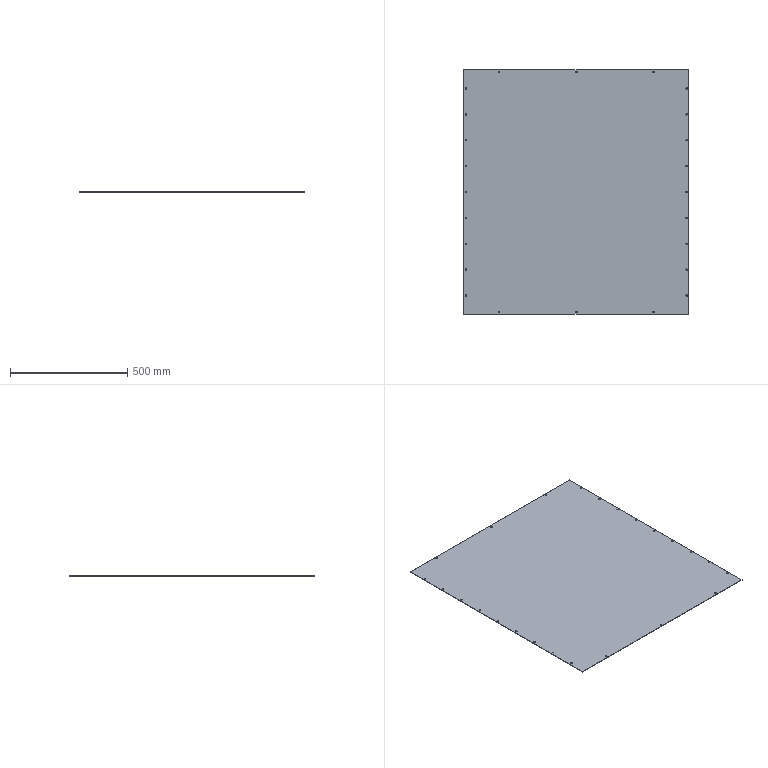Part | SolidWorks | 1 solid | 54 faces | box 959.5 x 1043 x 2 mm | volume 1999924 mm3 | cylinder 48 | plane 6 | commonest cylinder face diameters 6.5 x48